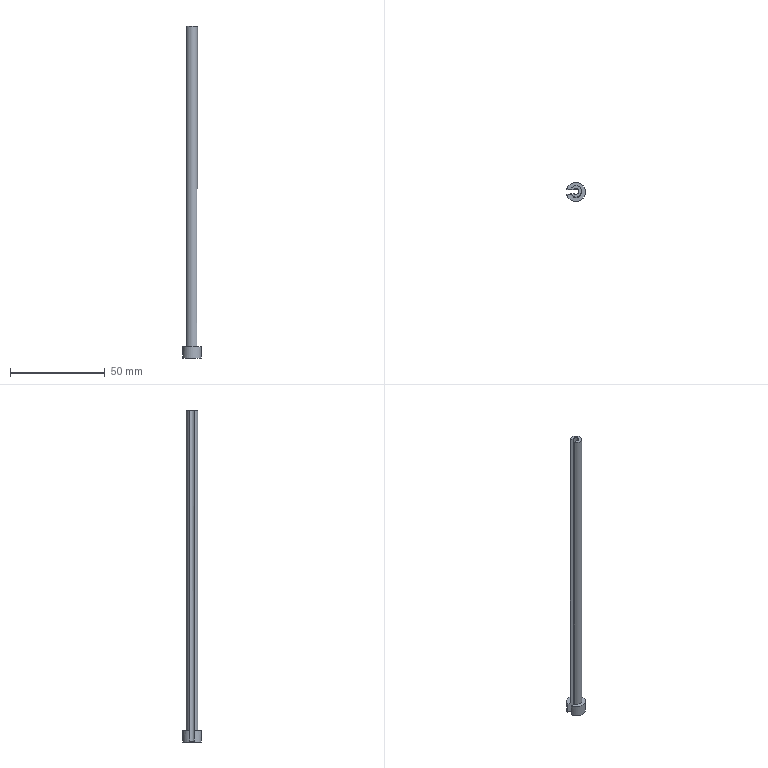Part | Creo | 1 solid | 11 faces | box 9.841 x 10 x 175.628 mm | volume 3287 mm3 | plane 7 | cylinder 3 | cone 1 | commonest cylinder face diameters 3 x1 6 x1 10 x1
STEP:
#1=CARTESIAN_POINT('',(-91.727,-41.75,-183.));
#2=VERTEX_POINT('',#1);
#3=CARTESIAN_POINT('',(-93.841,-41.75,-183.));
#4=VERTEX_POINT('',#3);
#5=CARTESIAN_POINT('',(-91.727,-41.75,-183.));
#6=DIRECTION('',(-1.,0.,0.));
#7=VECTOR('',#6,2.114);
#8=LINE('',#5,#7);
#9=EDGE_CURVE('',#2,#4,#8,.T.);
#10=ORIENTED_EDGE('',*,*,#9,.F.);
#11=CARTESIAN_POINT('',(-89.,-43.5,-183.));
#12=VERTEX_POINT('',#11);
#13=CARTESIAN_POINT('',(-89.,-40.5,-183.));
#14=DIRECTION('',(0.,0.,-1.));
#15=DIRECTION('',(0.,-1.,0.));
#16=AXIS2_PLACEMENT_3D('',#13,#14,#15);
#17=CIRCLE('',#16,3.);
#18=EDGE_CURVE('',#12,#2,#17,.T.);
#19=ORIENTED_EDGE('',*,*,#18,.F.);
#20=CARTESIAN_POINT('',(-89.,-37.5,-183.));
#21=VERTEX_POINT('',#20);
#22=CARTESIAN_POINT('',(-89.,-40.5,-183.));
#23=DIRECTION('',(0.,0.,-1.));
#24=DIRECTION('',(0.,1.,0.));
#25=AXIS2_PLACEMENT_3D('',#22,#23,#24);
#26=CIRCLE('',#25,3.);
#27=EDGE_CURVE('',#21,#12,#26,.T.);
#28=ORIENTED_EDGE('',*,*,#27,.F.);
#29=CARTESIAN_POINT('',(-91.727,-39.25,-183.));
#30=VERTEX_POINT('',#29);
#31=CARTESIAN_POINT('',(-89.,-40.5,-183.));
#32=DIRECTION('',(0.,0.,-1.));
#33=DIRECTION('',(-0.9091,0.4167,0.));
#34=AXIS2_PLACEMENT_3D('',#31,#32,#33);
#35=CIRCLE('',#34,3.);
#36=EDGE_CURVE('',#30,#21,#35,.T.);
#37=ORIENTED_EDGE('',*,*,#36,.F.);
#38=CARTESIAN_POINT('',(-93.841,-39.25,-183.));
#39=VERTEX_POINT('',#38);
#40=CARTESIAN_POINT('',(-93.841,-39.25,-183.));
#41=DIRECTION('',(1.,0.,0.));
#42=VECTOR('',#41,2.114);
#43=LINE('',#40,#42);
#44=EDGE_CURVE('',#39,#30,#43,.T.);
#45=ORIENTED_EDGE('',*,*,#44,.F.);
#46=CARTESIAN_POINT('',(-89.,-40.5,-183.));
#47=DIRECTION('',(0.,0.,1.));
#48=DIRECTION('',(-0.9682,-0.25,0.));
#49=AXIS2_PLACEMENT_3D('',#46,#47,#48);
#50=CIRCLE('',#49,5.);
#51=EDGE_CURVE('',#4,#39,#50,.T.);
#52=ORIENTED_EDGE('',*,*,#51,.F.);
#53=EDGE_LOOP('',(#10,#19,#28,#37,#45,#52));
#54=FACE_OUTER_BOUND('',#53,.F.);
#55=CARTESIAN_POINT('',(-89.,-40.5,-183.));
#56=DIRECTION('',(0.,0.,1.));
#57=DIRECTION('',(1.,0.,0.));
#58=AXIS2_PLACEMENT_3D('',#55,#56,#57);
#59=PLANE('',#58);
#60=ADVANCED_FACE('',(#54),#59,.T.);
#61=CARTESIAN_POINT('',(-89.829,-41.75,-188.5));
#62=VERTEX_POINT('',#61);
#63=CARTESIAN_POINT('',(-89.829,-41.75,-13.372));
#64=VERTEX_POINT('',#63);
#65=CARTESIAN_POINT('',(-89.829,-41.75,-188.5));
#66=DIRECTION('',(0.,0.,1.));
#67=VECTOR('',#66,175.128);
#68=LINE('',#65,#67);
#69=EDGE_CURVE('',#62,#64,#68,.T.);
#70=ORIENTED_EDGE('',*,*,#69,.T.);
#71=CARTESIAN_POINT('',(-91.727,-41.75,-13.372));
#72=VERTEX_POINT('',#71);
#73=CARTESIAN_POINT('',(-89.829,-41.75,-13.372));
#74=DIRECTION('',(-1.,0.,0.));
#75=VECTOR('',#74,1.898);
#76=LINE('',#73,#75);
#77=EDGE_CURVE('',#64,#72,#76,.T.);
#78=ORIENTED_EDGE('',*,*,#77,.T.);
#79=CARTESIAN_POINT('',(-91.727,-41.75,-13.372));
#80=DIRECTION('',(0.,0.,-1.));
#81=VECTOR('',#80,169.628);
#82=LINE('',#79,#81);
#83=EDGE_CURVE('',#72,#2,#82,.T.);
#84=ORIENTED_EDGE('',*,*,#83,.T.);
#85=ORIENTED_EDGE('',*,*,#9,.T.);
#86=CARTESIAN_POINT('',(-93.841,-41.75,-188.5));
#87=VERTEX_POINT('',#86);
#88=CARTESIAN_POINT('',(-93.841,-41.75,-183.));
#89=DIRECTION('',(0.,0.,-1.));
#90=VECTOR('',#89,5.5);
#91=LINE('',#88,#90);
#92=EDGE_CURVE('',#4,#87,#91,.T.);
#93=ORIENTED_EDGE('',*,*,#92,.T.);
#94=CARTESIAN_POINT('',(-93.841,-41.75,-188.5));
#95=DIRECTION('',(1.,0.,0.));
#96=VECTOR('',#95,4.012);
#97=LINE('',#94,#96);
#98=EDGE_CURVE('',#87,#62,#97,.T.);
#99=ORIENTED_EDGE('',*,*,#98,.T.);
#100=EDGE_LOOP('',(#70,#78,#84,#85,#93,#99));
#101=FACE_OUTER_BOUND('',#100,.F.);
#102=CARTESIAN_POINT('',(-89.,-41.75,-4.872));
#103=DIRECTION('',(0.,-1.,0.));
#104=DIRECTION('',(0.,0.,1.));
#105=AXIS2_PLACEMENT_3D('',#102,#103,#104);
#106=PLANE('',#105);
#107=ADVANCED_FACE('',(#101),#106,.F.);
#108=CARTESIAN_POINT('',(-89.829,-39.25,-13.372));
#109=VERTEX_POINT('',#108);
#110=CARTESIAN_POINT('',(-89.829,-39.25,-188.5));
#111=VERTEX_POINT('',#110);
#112=CARTESIAN_POINT('',(-89.829,-39.25,-13.372));
#113=DIRECTION('',(0.,0.,-1.));
#114=VECTOR('',#113,175.128);
#115=LINE('',#112,#114);
#116=EDGE_CURVE('',#109,#111,#115,.T.);
#117=ORIENTED_EDGE('',*,*,#116,.F.);
#118=CARTESIAN_POINT('',(-89.,-39.,-13.372));
#119=VERTEX_POINT('',#118);
#120=CARTESIAN_POINT('',(-89.,-40.5,-13.372));
#121=DIRECTION('',(0.,0.,-1.));
#122=DIRECTION('',(-0.5528,0.8333,0.));
#123=AXIS2_PLACEMENT_3D('',#120,#121,#122);
#124=CIRCLE('',#123,1.5);
#125=EDGE_CURVE('',#109,#119,#124,.T.);
#126=ORIENTED_EDGE('',*,*,#125,.T.);
#127=CARTESIAN_POINT('',(-89.,-42.,-13.372));
#128=VERTEX_POINT('',#127);
#129=CARTESIAN_POINT('',(-89.,-40.5,-13.372));
#130=DIRECTION('',(0.,0.,-1.));
#131=DIRECTION('',(0.,1.,0.));
#132=AXIS2_PLACEMENT_3D('',#129,#130,#131);
#133=CIRCLE('',#132,1.5);
#134=EDGE_CURVE('',#119,#128,#133,.T.);
#135=ORIENTED_EDGE('',*,*,#134,.T.);
#136=CARTESIAN_POINT('',(-89.,-40.5,-13.372));
#137=DIRECTION('',(0.,0.,-1.));
#138=DIRECTION('',(0.,-1.,0.));
#139=AXIS2_PLACEMENT_3D('',#136,#137,#138);
#140=CIRCLE('',#139,1.5);
#141=EDGE_CURVE('',#128,#64,#140,.T.);
#142=ORIENTED_EDGE('',*,*,#141,.T.);
#143=ORIENTED_EDGE('',*,*,#69,.F.);
#144=CARTESIAN_POINT('',(-89.,-42.,-188.5));
#145=VERTEX_POINT('',#144);
#146=CARTESIAN_POINT('',(-89.,-40.5,-188.5));
#147=DIRECTION('',(0.,0.,1.));
#148=DIRECTION('',(-0.5528,-0.8333,0.));
#149=AXIS2_PLACEMENT_3D('',#146,#147,#148);
#150=CIRCLE('',#149,1.5);
#151=EDGE_CURVE('',#62,#145,#150,.T.);
#152=ORIENTED_EDGE('',*,*,#151,.T.);
#153=CARTESIAN_POINT('',(-87.5,-40.5,-188.5));
#154=VERTEX_POINT('',#153);
#155=CARTESIAN_POINT('',(-89.,-40.5,-188.5));
#156=DIRECTION('',(0.,0.,1.));
#157=DIRECTION('',(0.,-1.,0.));
#158=AXIS2_PLACEMENT_3D('',#155,#156,#157);
#159=CIRCLE('',#158,1.5);
#160=EDGE_CURVE('',#145,#154,#159,.T.);
#161=ORIENTED_EDGE('',*,*,#160,.T.);
#162=CARTESIAN_POINT('',(-89.,-39.,-188.5));
#163=VERTEX_POINT('',#162);
#164=CARTESIAN_POINT('',(-89.,-40.5,-188.5));
#165=DIRECTION('',(0.,0.,1.));
#166=DIRECTION('',(1.,0.,0.));
#167=AXIS2_PLACEMENT_3D('',#164,#165,#166);
#168=CIRCLE('',#167,1.5);
#169=EDGE_CURVE('',#154,#163,#168,.T.);
#170=ORIENTED_EDGE('',*,*,#169,.T.);
#171=CARTESIAN_POINT('',(-89.,-40.5,-188.5));
#172=DIRECTION('',(0.,0.,1.));
#173=DIRECTION('',(0.,1.,0.));
#174=AXIS2_PLACEMENT_3D('',#171,#172,#173);
#175=CIRCLE('',#174,1.5);
#176=EDGE_CURVE('',#163,#111,#175,.T.);
#177=ORIENTED_EDGE('',*,*,#176,.T.);
#178=EDGE_LOOP('',(#117,#126,#135,#142,#143,#152,#161,#170,#177));
#179=FACE_OUTER_BOUND('',#178,.F.);
#180=CARTESIAN_POINT('',(-89.,-40.5,-1.372));
#181=DIRECTION('',(0.,0.,-1.));
#182=DIRECTION('',(0.,1.,0.));
#183=AXIS2_PLACEMENT_3D('',#180,#181,#182);
#184=CYLINDRICAL_SURFACE('',#183,1.5);
#185=ADVANCED_FACE('',(#179),#184,.F.);
#186=CARTESIAN_POINT('',(-93.841,-39.25,-188.5));
#187=VERTEX_POINT('',#186);
#188=CARTESIAN_POINT('',(-93.841,-39.25,-188.5));
#189=DIRECTION('',(0.,0.,1.));
#190=VECTOR('',#189,5.5);
#191=LINE('',#188,#190);
#192=EDGE_CURVE('',#187,#39,#191,.T.);
#193=ORIENTED_EDGE('',*,*,#192,.T.);
#194=ORIENTED_EDGE('',*,*,#44,.T.);
#195=CARTESIAN_POINT('',(-91.727,-39.25,-13.372));
#196=VERTEX_POINT('',#195);
#197=CARTESIAN_POINT('',(-91.727,-39.25,-183.));
#198=DIRECTION('',(0.,0.,1.));
#199=VECTOR('',#198,169.628);
#200=LINE('',#197,#199);
#201=EDGE_CURVE('',#30,#196,#200,.T.);
#202=ORIENTED_EDGE('',*,*,#201,.T.);
#203=CARTESIAN_POINT('',(-89.829,-39.25,-13.372));
#204=DIRECTION('',(-1.,0.,0.));
#205=VECTOR('',#204,1.898);
#206=LINE('',#203,#205);
#207=EDGE_CURVE('',#109,#196,#206,.T.);
#208=ORIENTED_EDGE('',*,*,#207,.F.);
#209=ORIENTED_EDGE('',*,*,#116,.T.);
#210=CARTESIAN_POINT('',(-89.829,-39.25,-188.5));
#211=DIRECTION('',(-1.,0.,0.));
#212=VECTOR('',#211,4.012);
#213=LINE('',#210,#212);
#214=EDGE_CURVE('',#111,#187,#213,.T.);
#215=ORIENTED_EDGE('',*,*,#214,.T.);
#216=EDGE_LOOP('',(#193,#194,#202,#208,#209,#215));
#217=FACE_OUTER_BOUND('',#216,.F.);
#218=CARTESIAN_POINT('',(-89.,-39.25,-74.872));
#219=DIRECTION('',(0.,1.,0.));
#220=DIRECTION('',(0.,0.,-1.));
#221=AXIS2_PLACEMENT_3D('',#218,#219,#220);
#222=PLANE('',#221);
#223=ADVANCED_FACE('',(#217),#222,.F.);
#224=CARTESIAN_POINT('',(-84.,-40.5,-189.));
#225=VERTEX_POINT('',#224);
#226=CARTESIAN_POINT('',(-93.684,-42.25,-189.));
#227=VERTEX_POINT('',#226);
#228=CARTESIAN_POINT('',(-89.,-40.5,-189.));
#229=DIRECTION('',(0.,0.,-1.));
#230=DIRECTION('',(1.,0.,0.));
#231=AXIS2_PLACEMENT_3D('',#228,#229,#230);
#232=CIRCLE('',#231,5.);
#233=EDGE_CURVE('',#225,#227,#232,.T.);
#234=ORIENTED_EDGE('',*,*,#233,.T.);
#235=CARTESIAN_POINT('',(-93.684,-42.25,-189.));
#236=CARTESIAN_POINT('',(-93.745,-42.085,-188.835));
#237=CARTESIAN_POINT('',(-93.798,-41.918,-188.668));
#238=CARTESIAN_POINT('',(-93.841,-41.75,-188.5));
#239=B_SPLINE_CURVE_WITH_KNOTS('',3,(#235,#236,#237,#238),.UNSPECIFIED.,.F.,.F.,(4,4),(0.,1.),.UNSPECIFIED.);
#240=EDGE_CURVE('',#227,#87,#239,.T.);
#241=ORIENTED_EDGE('',*,*,#240,.T.);
#242=ORIENTED_EDGE('',*,*,#92,.F.);
#243=ORIENTED_EDGE('',*,*,#51,.T.);
#244=ORIENTED_EDGE('',*,*,#192,.F.);
#245=CARTESIAN_POINT('',(-93.684,-38.75,-189.));
#246=VERTEX_POINT('',#245);
#247=CARTESIAN_POINT('',(-93.841,-39.25,-188.5));
#248=CARTESIAN_POINT('',(-93.798,-39.082,-188.668));
#249=CARTESIAN_POINT('',(-93.745,-38.915,-188.835));
#250=CARTESIAN_POINT('',(-93.684,-38.75,-189.));
#251=B_SPLINE_CURVE_WITH_KNOTS('',3,(#247,#248,#249,#250),.UNSPECIFIED.,.F.,.F.,(4,4),(0.,1.),.UNSPECIFIED.);
#252=EDGE_CURVE('',#187,#246,#251,.T.);
#253=ORIENTED_EDGE('',*,*,#252,.T.);
#254=CARTESIAN_POINT('',(-89.,-40.5,-189.));
#255=DIRECTION('',(0.,0.,-1.));
#256=DIRECTION('',(-0.9367,0.35,0.));
#257=AXIS2_PLACEMENT_3D('',#254,#255,#256);
#258=CIRCLE('',#257,5.);
#259=EDGE_CURVE('',#246,#225,#258,.T.);
#260=ORIENTED_EDGE('',*,*,#259,.T.);
#261=EDGE_LOOP('',(#234,#241,#242,#243,#244,#253,#260));
#262=FACE_OUTER_BOUND('',#261,.F.);
#263=CARTESIAN_POINT('',(-89.,-40.5,-183.));
#264=DIRECTION('',(0.,0.,-1.));
#265=DIRECTION('',(-1.,0.,0.));
#266=AXIS2_PLACEMENT_3D('',#263,#264,#265);
#267=CYLINDRICAL_SURFACE('',#266,5.);
#268=ADVANCED_FACE('',(#262),#267,.T.);
#269=CARTESIAN_POINT('',(-89.968,-42.25,-189.));
#270=VERTEX_POINT('',#269);
#271=CARTESIAN_POINT('',(-87.,-40.5,-189.));
#272=VERTEX_POINT('',#271);
#273=CARTESIAN_POINT('',(-89.,-40.5,-189.));
#274=DIRECTION('',(0.,0.,1.));
#275=DIRECTION('',(-0.4841,-0.875,0.));
#276=AXIS2_PLACEMENT_3D('',#273,#274,#275);
#277=CIRCLE('',#276,2.);
#278=EDGE_CURVE('',#270,#272,#277,.T.);
#279=ORIENTED_EDGE('',*,*,#278,.F.);
#280=CARTESIAN_POINT('',(-89.968,-42.25,-189.));
#281=DIRECTION('',(-1.,0.,0.));
#282=VECTOR('',#281,3.716);
#283=LINE('',#280,#282);
#284=EDGE_CURVE('',#270,#227,#283,.T.);
#285=ORIENTED_EDGE('',*,*,#284,.T.);
#286=ORIENTED_EDGE('',*,*,#233,.F.);
#287=ORIENTED_EDGE('',*,*,#259,.F.);
#288=CARTESIAN_POINT('',(-89.968,-38.75,-189.));
#289=VERTEX_POINT('',#288);
#290=CARTESIAN_POINT('',(-93.684,-38.75,-189.));
#291=DIRECTION('',(1.,0.,0.));
#292=VECTOR('',#291,3.716);
#293=LINE('',#290,#292);
#294=EDGE_CURVE('',#246,#289,#293,.T.);
#295=ORIENTED_EDGE('',*,*,#294,.T.);
#296=CARTESIAN_POINT('',(-89.,-40.5,-189.));
#297=DIRECTION('',(0.,0.,1.));
#298=DIRECTION('',(1.,0.,0.));
#299=AXIS2_PLACEMENT_3D('',#296,#297,#298);
#300=CIRCLE('',#299,2.);
#301=EDGE_CURVE('',#272,#289,#300,.T.);
#302=ORIENTED_EDGE('',*,*,#301,.F.);
#303=EDGE_LOOP('',(#279,#285,#286,#287,#295,#302));
#304=FACE_OUTER_BOUND('',#303,.F.);
#305=CARTESIAN_POINT('',(-89.,-40.5,-189.));
#306=DIRECTION('',(0.,0.,-1.));
#307=DIRECTION('',(-1.,0.,0.));
#308=AXIS2_PLACEMENT_3D('',#305,#306,#307);
#309=PLANE('',#308);
#310=ADVANCED_FACE('',(#304),#309,.T.);
#311=CARTESIAN_POINT('',(-89.829,-41.75,-188.5));
#312=CARTESIAN_POINT('',(-89.846,-41.805,-188.555));
#313=CARTESIAN_POINT('',(-89.878,-41.916,-188.666));
#314=CARTESIAN_POINT('',(-89.925,-42.083,-188.833));
#315=CARTESIAN_POINT('',(-89.954,-42.194,-188.944));
#316=CARTESIAN_POINT('',(-89.968,-42.25,-189.));
#317=B_SPLINE_CURVE_WITH_KNOTS('',3,(#311,#312,#313,#314,#315,#316),.UNSPECIFIED.,.F.,.F.,(4,1,1,4),(0.,0.3333,0.6667,1.),.UNSPECIFIED.);
#318=EDGE_CURVE('',#62,#270,#317,.T.);
#319=ORIENTED_EDGE('',*,*,#318,.T.);
#320=ORIENTED_EDGE('',*,*,#278,.T.);
#321=ORIENTED_EDGE('',*,*,#301,.T.);
#322=CARTESIAN_POINT('',(-89.829,-39.25,-188.5));
#323=CARTESIAN_POINT('',(-89.845,-39.196,-188.554));
#324=CARTESIAN_POINT('',(-89.877,-39.087,-188.663));
#325=CARTESIAN_POINT('',(-89.924,-38.921,-188.829));
#326=CARTESIAN_POINT('',(-89.953,-38.807,-188.943));
#327=CARTESIAN_POINT('',(-89.968,-38.75,-189.));
#328=B_SPLINE_CURVE_WITH_KNOTS('',3,(#322,#323,#324,#325,#326,#327),.UNSPECIFIED.,.F.,.F.,(4,1,1,4),(0.,0.3333,0.6667,1.),.UNSPECIFIED.);
#329=EDGE_CURVE('',#111,#289,#328,.T.);
#330=ORIENTED_EDGE('',*,*,#329,.F.);
#331=ORIENTED_EDGE('',*,*,#176,.F.);
#332=ORIENTED_EDGE('',*,*,#169,.F.);
#333=ORIENTED_EDGE('',*,*,#160,.F.);
#334=ORIENTED_EDGE('',*,*,#151,.F.);
#335=EDGE_LOOP('',(#319,#320,#321,#330,#331,#332,#333,#334));
#336=FACE_OUTER_BOUND('',#335,.F.);
#337=CARTESIAN_POINT('',(-89.,-40.5,-188.75));
#338=DIRECTION('',(0.,0.,-1.));
#339=DIRECTION('',(-1.,0.,0.));
#340=AXIS2_PLACEMENT_3D('',#337,#338,#339);
#341=CONICAL_SURFACE('',#340,1.75,45.);
#342=ADVANCED_FACE('',(#336),#341,.F.);
#343=ORIENTED_EDGE('',*,*,#240,.F.);
#344=ORIENTED_EDGE('',*,*,#284,.F.);
#345=ORIENTED_EDGE('',*,*,#318,.F.);
#346=ORIENTED_EDGE('',*,*,#98,.F.);
#347=EDGE_LOOP('',(#343,#344,#345,#346));
#348=FACE_OUTER_BOUND('',#347,.F.);
#349=CARTESIAN_POINT('',(-89.,-41.75,-188.5));
#350=DIRECTION('',(0.,0.7071,-0.7071));
#351=DIRECTION('',(1.,0.,0.));
#352=AXIS2_PLACEMENT_3D('',#349,#350,#351);
#353=PLANE('',#352);
#354=ADVANCED_FACE('',(#348),#353,.T.);
#355=ORIENTED_EDGE('',*,*,#252,.F.);
#356=ORIENTED_EDGE('',*,*,#214,.F.);
#357=ORIENTED_EDGE('',*,*,#329,.T.);
#358=ORIENTED_EDGE('',*,*,#294,.F.);
#359=EDGE_LOOP('',(#355,#356,#357,#358));
#360=FACE_OUTER_BOUND('',#359,.F.);
#361=CARTESIAN_POINT('',(-89.,-39.25,-188.5));
#362=DIRECTION('',(0.,-0.7071,-0.7071));
#363=DIRECTION('',(-1.,0.,0.));
#364=AXIS2_PLACEMENT_3D('',#361,#362,#363);
#365=PLANE('',#364);
#366=ADVANCED_FACE('',(#360),#365,.T.);
#367=ORIENTED_EDGE('',*,*,#18,.T.);
#368=ORIENTED_EDGE('',*,*,#83,.F.);
#369=CARTESIAN_POINT('',(-89.,-43.5,-13.372));
#370=VERTEX_POINT('',#369);
#371=CARTESIAN_POINT('',(-89.,-40.5,-13.372));
#372=DIRECTION('',(0.,0.,1.));
#373=DIRECTION('',(-0.9091,-0.4167,0.));
#374=AXIS2_PLACEMENT_3D('',#371,#372,#373);
#375=CIRCLE('',#374,3.);
#376=EDGE_CURVE('',#72,#370,#375,.T.);
#377=ORIENTED_EDGE('',*,*,#376,.T.);
#378=CARTESIAN_POINT('',(-86.,-40.5,-13.372));
#379=VERTEX_POINT('',#378);
#380=CARTESIAN_POINT('',(-89.,-40.5,-13.372));
#381=DIRECTION('',(0.,0.,1.));
#382=DIRECTION('',(0.,-1.,0.));
#383=AXIS2_PLACEMENT_3D('',#380,#381,#382);
#384=CIRCLE('',#383,3.);
#385=EDGE_CURVE('',#370,#379,#384,.T.);
#386=ORIENTED_EDGE('',*,*,#385,.T.);
#387=CARTESIAN_POINT('',(-89.,-37.5,-13.372));
#388=VERTEX_POINT('',#387);
#389=CARTESIAN_POINT('',(-89.,-40.5,-13.372));
#390=DIRECTION('',(0.,0.,1.));
#391=DIRECTION('',(1.,0.,0.));
#392=AXIS2_PLACEMENT_3D('',#389,#390,#391);
#393=CIRCLE('',#392,3.);
#394=EDGE_CURVE('',#379,#388,#393,.T.);
#395=ORIENTED_EDGE('',*,*,#394,.T.);
#396=CARTESIAN_POINT('',(-89.,-40.5,-13.372));
#397=DIRECTION('',(0.,0.,1.));
#398=DIRECTION('',(0.,1.,0.));
#399=AXIS2_PLACEMENT_3D('',#396,#397,#398);
#400=CIRCLE('',#399,3.);
#401=EDGE_CURVE('',#388,#196,#400,.T.);
#402=ORIENTED_EDGE('',*,*,#401,.T.);
#403=ORIENTED_EDGE('',*,*,#201,.F.);
#404=ORIENTED_EDGE('',*,*,#36,.T.);
#405=ORIENTED_EDGE('',*,*,#27,.T.);
#406=EDGE_LOOP('',(#367,#368,#377,#386,#395,#402,#403,#404,#405));
#407=FACE_OUTER_BOUND('',#406,.F.);
#408=CARTESIAN_POINT('',(-89.,-40.5,-1.372));
#409=DIRECTION('',(0.,0.,-1.));
#410=DIRECTION('',(0.,1.,0.));
#411=AXIS2_PLACEMENT_3D('',#408,#409,#410);
#412=CYLINDRICAL_SURFACE('',#411,3.);
#413=ADVANCED_FACE('',(#407),#412,.T.);
#414=ORIENTED_EDGE('',*,*,#376,.F.);
#415=ORIENTED_EDGE('',*,*,#77,.F.);
#416=ORIENTED_EDGE('',*,*,#141,.F.);
#417=ORIENTED_EDGE('',*,*,#134,.F.);
#418=ORIENTED_EDGE('',*,*,#125,.F.);
#419=ORIENTED_EDGE('',*,*,#207,.T.);
#420=ORIENTED_EDGE('',*,*,#401,.F.);
#421=ORIENTED_EDGE('',*,*,#394,.F.);
#422=ORIENTED_EDGE('',*,*,#385,.F.);
#423=EDGE_LOOP('',(#414,#415,#416,#417,#418,#419,#420,#421,#422));
#424=FACE_OUTER_BOUND('',#423,.F.);
#425=CARTESIAN_POINT('',(-89.,-40.5,-13.372));
#426=DIRECTION('',(0.,0.,-1.));
#427=DIRECTION('',(0.,1.,0.));
#428=AXIS2_PLACEMENT_3D('',#425,#426,#427);
#429=PLANE('',#428);
#430=ADVANCED_FACE('',(#424),#429,.F.);
#431=CLOSED_SHELL('',(#60,#107,#185,#223,#268,#310,#342,#354,#366,#413,#430));
#432=MANIFOLD_SOLID_BREP('',#431);
#433=(LENGTH_UNIT()NAMED_UNIT(*)SI_UNIT(.MILLI.,.METRE.));
#434=UNCERTAINTY_MEASURE_WITH_UNIT(LENGTH_MEASURE(0.01762),#433,'','');
#435=(NAMED_UNIT(*)PLANE_ANGLE_UNIT()SI_UNIT($,.RADIAN.));
#436=PLANE_ANGLE_MEASURE_WITH_UNIT(PLANE_ANGLE_MEASURE(0.01745),#435);
#437=(CONVERSION_BASED_UNIT('DEGREE',#436)NAMED_UNIT(*)PLANE_ANGLE_UNIT());
#438=(NAMED_UNIT(*)SI_UNIT($,.STERADIAN.)SOLID_ANGLE_UNIT());
#439=(GEOMETRIC_REPRESENTATION_CONTEXT(3)GLOBAL_UNCERTAINTY_ASSIGNED_CONTEXT((#434))GLOBAL_UNIT_ASSIGNED_CONTEXT((#433,#437,#438))REPRESENTATION_CONTEXT('',''));
#440=ADVANCED_BREP_SHAPE_REPRESENTATION('',(#432),#439);